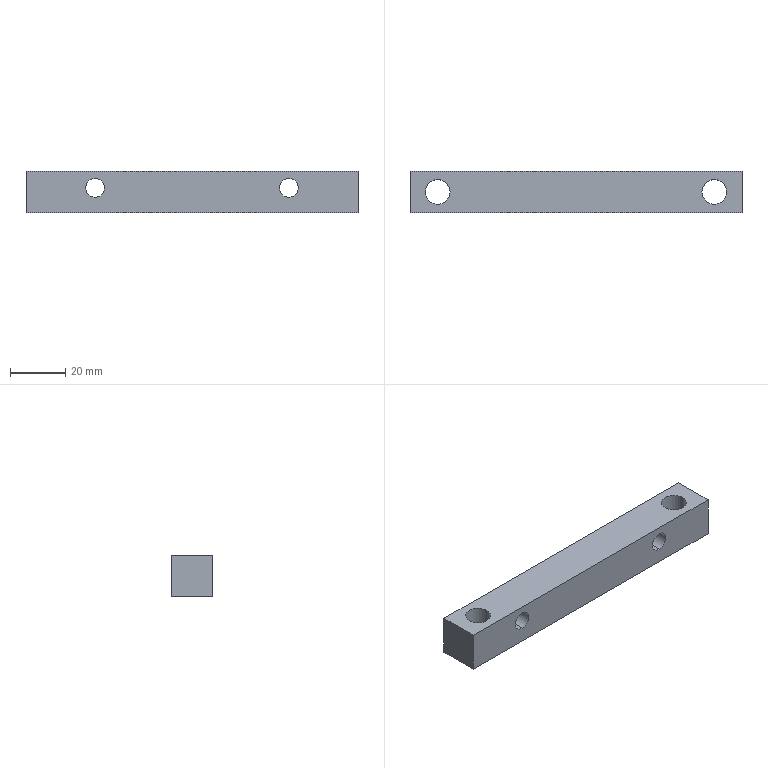Part | SolidWorks | features BaseBody 1 | 1 solid | 14 faces | box 120 x 15 x 15 mm | volume 24002 mm3 | cylinder 8 | plane 6 | commonest cylinder face diameters 6.8 x4 9 x4
STEP:
#1=CARTESIAN_POINT('',(-35.,7.5,12.4));
#2=VERTEX_POINT('',#1);
#3=CARTESIAN_POINT('',(-35.,7.5,5.6));
#4=VERTEX_POINT('',#3);
#5=CARTESIAN_POINT('',(-35.,7.5,9.));
#6=DIRECTION('',(0.,-1.,0.));
#7=DIRECTION('',(0.,0.,-1.));
#8=AXIS2_PLACEMENT_3D('',#5,#6,#7);
#9=CIRCLE('',#8,3.4);
#10=EDGE_CURVE('',#2,#4,#9,.T.);
#11=ORIENTED_EDGE('',*,*,#10,.F.);
#12=CARTESIAN_POINT('',(-35.,-7.5,12.4));
#13=VERTEX_POINT('',#12);
#14=CARTESIAN_POINT('',(-35.,-7.5,12.4));
#15=DIRECTION('',(0.,-1.,0.));
#16=VECTOR('',#15,1000.);
#17=LINE('',#14,#16);
#18=EDGE_CURVE('',#2,#13,#17,.T.);
#19=ORIENTED_EDGE('',*,*,#18,.T.);
#20=CARTESIAN_POINT('',(-35.,-7.5,5.6));
#21=VERTEX_POINT('',#20);
#22=CARTESIAN_POINT('',(-35.,-7.5,9.));
#23=DIRECTION('',(0.,-1.,0.));
#24=DIRECTION('',(0.,0.,-1.));
#25=AXIS2_PLACEMENT_3D('',#22,#23,#24);
#26=CIRCLE('',#25,3.4);
#27=EDGE_CURVE('',#13,#21,#26,.T.);
#28=ORIENTED_EDGE('',*,*,#27,.T.);
#29=CARTESIAN_POINT('',(-35.,-7.5,5.6));
#30=DIRECTION('',(0.,-1.,0.));
#31=VECTOR('',#30,1000.);
#32=LINE('',#29,#31);
#33=EDGE_CURVE('',#4,#21,#32,.T.);
#34=ORIENTED_EDGE('',*,*,#33,.F.);
#35=EDGE_LOOP('',(#11,#19,#28,#34));
#36=FACE_OUTER_BOUND('',#35,.T.);
#37=CARTESIAN_POINT('',(-35.,-7.5,9.));
#38=DIRECTION('',(0.,-1.,0.));
#39=DIRECTION('',(0.,0.,-1.));
#40=AXIS2_PLACEMENT_3D('',#37,#38,#39);
#41=CYLINDRICAL_SURFACE('',#40,3.4);
#42=ADVANCED_FACE('',(#36),#41,.F.);
#43=CARTESIAN_POINT('',(35.,7.5,12.4));
#44=VERTEX_POINT('',#43);
#45=CARTESIAN_POINT('',(35.,7.5,5.6));
#46=VERTEX_POINT('',#45);
#47=CARTESIAN_POINT('',(35.,7.5,9.));
#48=DIRECTION('',(0.,-1.,0.));
#49=DIRECTION('',(0.,0.,-1.));
#50=AXIS2_PLACEMENT_3D('',#47,#48,#49);
#51=CIRCLE('',#50,3.4);
#52=EDGE_CURVE('',#44,#46,#51,.T.);
#53=ORIENTED_EDGE('',*,*,#52,.F.);
#54=CARTESIAN_POINT('',(35.,-7.5,12.4));
#55=VERTEX_POINT('',#54);
#56=CARTESIAN_POINT('',(35.,-7.5,12.4));
#57=DIRECTION('',(0.,-1.,0.));
#58=VECTOR('',#57,1000.);
#59=LINE('',#56,#58);
#60=EDGE_CURVE('',#44,#55,#59,.T.);
#61=ORIENTED_EDGE('',*,*,#60,.T.);
#62=CARTESIAN_POINT('',(35.,-7.5,5.6));
#63=VERTEX_POINT('',#62);
#64=CARTESIAN_POINT('',(35.,-7.5,9.));
#65=DIRECTION('',(0.,-1.,0.));
#66=DIRECTION('',(0.,0.,-1.));
#67=AXIS2_PLACEMENT_3D('',#64,#65,#66);
#68=CIRCLE('',#67,3.4);
#69=EDGE_CURVE('',#55,#63,#68,.T.);
#70=ORIENTED_EDGE('',*,*,#69,.T.);
#71=CARTESIAN_POINT('',(35.,-7.5,5.6));
#72=DIRECTION('',(0.,-1.,0.));
#73=VECTOR('',#72,1000.);
#74=LINE('',#71,#73);
#75=EDGE_CURVE('',#46,#63,#74,.T.);
#76=ORIENTED_EDGE('',*,*,#75,.F.);
#77=EDGE_LOOP('',(#53,#61,#70,#76));
#78=FACE_OUTER_BOUND('',#77,.T.);
#79=CARTESIAN_POINT('',(35.,-7.5,9.));
#80=DIRECTION('',(0.,-1.,0.));
#81=DIRECTION('',(0.,0.,-1.));
#82=AXIS2_PLACEMENT_3D('',#79,#80,#81);
#83=CYLINDRICAL_SURFACE('',#82,3.4);
#84=ADVANCED_FACE('',(#78),#83,.F.);
#85=CARTESIAN_POINT('',(-54.5,0.,0.));
#86=VERTEX_POINT('',#85);
#87=CARTESIAN_POINT('',(-45.5,0.,0.));
#88=VERTEX_POINT('',#87);
#89=CARTESIAN_POINT('',(-50.,0.,0.));
#90=DIRECTION('',(0.,0.,1.));
#91=DIRECTION('',(1.,0.,0.));
#92=AXIS2_PLACEMENT_3D('',#89,#90,#91);
#93=CIRCLE('',#92,4.5);
#94=EDGE_CURVE('',#86,#88,#93,.T.);
#95=ORIENTED_EDGE('',*,*,#94,.F.);
#96=CARTESIAN_POINT('',(-54.5,0.,15.));
#97=VERTEX_POINT('',#96);
#98=CARTESIAN_POINT('',(-54.5,0.,15.));
#99=DIRECTION('',(0.,0.,1.));
#100=VECTOR('',#99,1000.);
#101=LINE('',#98,#100);
#102=EDGE_CURVE('',#86,#97,#101,.T.);
#103=ORIENTED_EDGE('',*,*,#102,.T.);
#104=CARTESIAN_POINT('',(-45.5,0.,15.));
#105=VERTEX_POINT('',#104);
#106=CARTESIAN_POINT('',(-50.,0.,15.));
#107=DIRECTION('',(0.,0.,1.));
#108=DIRECTION('',(1.,0.,0.));
#109=AXIS2_PLACEMENT_3D('',#106,#107,#108);
#110=CIRCLE('',#109,4.5);
#111=EDGE_CURVE('',#97,#105,#110,.T.);
#112=ORIENTED_EDGE('',*,*,#111,.T.);
#113=CARTESIAN_POINT('',(-45.5,0.,15.));
#114=DIRECTION('',(0.,0.,1.));
#115=VECTOR('',#114,1000.);
#116=LINE('',#113,#115);
#117=EDGE_CURVE('',#88,#105,#116,.T.);
#118=ORIENTED_EDGE('',*,*,#117,.F.);
#119=EDGE_LOOP('',(#95,#103,#112,#118));
#120=FACE_OUTER_BOUND('',#119,.T.);
#121=CARTESIAN_POINT('',(-50.,0.,15.));
#122=DIRECTION('',(0.,0.,1.));
#123=DIRECTION('',(1.,0.,0.));
#124=AXIS2_PLACEMENT_3D('',#121,#122,#123);
#125=CYLINDRICAL_SURFACE('',#124,4.5);
#126=ADVANCED_FACE('',(#120),#125,.F.);
#127=CARTESIAN_POINT('',(45.5,0.,0.));
#128=VERTEX_POINT('',#127);
#129=CARTESIAN_POINT('',(54.5,0.,0.));
#130=VERTEX_POINT('',#129);
#131=CARTESIAN_POINT('',(50.,0.,0.));
#132=DIRECTION('',(0.,0.,1.));
#133=DIRECTION('',(1.,0.,0.));
#134=AXIS2_PLACEMENT_3D('',#131,#132,#133);
#135=CIRCLE('',#134,4.5);
#136=EDGE_CURVE('',#128,#130,#135,.T.);
#137=ORIENTED_EDGE('',*,*,#136,.F.);
#138=CARTESIAN_POINT('',(45.5,0.,15.));
#139=VERTEX_POINT('',#138);
#140=CARTESIAN_POINT('',(45.5,0.,15.));
#141=DIRECTION('',(0.,0.,1.));
#142=VECTOR('',#141,1000.);
#143=LINE('',#140,#142);
#144=EDGE_CURVE('',#128,#139,#143,.T.);
#145=ORIENTED_EDGE('',*,*,#144,.T.);
#146=CARTESIAN_POINT('',(54.5,0.,15.));
#147=VERTEX_POINT('',#146);
#148=CARTESIAN_POINT('',(50.,0.,15.));
#149=DIRECTION('',(0.,0.,1.));
#150=DIRECTION('',(1.,0.,0.));
#151=AXIS2_PLACEMENT_3D('',#148,#149,#150);
#152=CIRCLE('',#151,4.5);
#153=EDGE_CURVE('',#139,#147,#152,.T.);
#154=ORIENTED_EDGE('',*,*,#153,.T.);
#155=CARTESIAN_POINT('',(54.5,0.,15.));
#156=DIRECTION('',(0.,0.,1.));
#157=VECTOR('',#156,1000.);
#158=LINE('',#155,#157);
#159=EDGE_CURVE('',#130,#147,#158,.T.);
#160=ORIENTED_EDGE('',*,*,#159,.F.);
#161=EDGE_LOOP('',(#137,#145,#154,#160));
#162=FACE_OUTER_BOUND('',#161,.T.);
#163=CARTESIAN_POINT('',(50.,0.,15.));
#164=DIRECTION('',(0.,0.,1.));
#165=DIRECTION('',(1.,0.,0.));
#166=AXIS2_PLACEMENT_3D('',#163,#164,#165);
#167=CYLINDRICAL_SURFACE('',#166,4.5);
#168=ADVANCED_FACE('',(#162),#167,.F.);
#169=CARTESIAN_POINT('',(60.,-7.5,0.));
#170=VERTEX_POINT('',#169);
#171=CARTESIAN_POINT('',(60.,7.5,0.));
#172=VERTEX_POINT('',#171);
#173=CARTESIAN_POINT('',(60.,7.5,0.));
#174=DIRECTION('',(0.,1.,0.));
#175=VECTOR('',#174,1000.);
#176=LINE('',#173,#175);
#177=EDGE_CURVE('',#170,#172,#176,.T.);
#178=ORIENTED_EDGE('',*,*,#177,.T.);
#179=CARTESIAN_POINT('',(60.,7.5,15.));
#180=VERTEX_POINT('',#179);
#181=CARTESIAN_POINT('',(60.,7.5,15.));
#182=DIRECTION('',(0.,0.,-1.));
#183=VECTOR('',#182,1000.);
#184=LINE('',#181,#183);
#185=EDGE_CURVE('',#180,#172,#184,.T.);
#186=ORIENTED_EDGE('',*,*,#185,.F.);
#187=CARTESIAN_POINT('',(60.,-7.5,15.));
#188=VERTEX_POINT('',#187);
#189=CARTESIAN_POINT('',(60.,7.5,15.));
#190=DIRECTION('',(0.,1.,0.));
#191=VECTOR('',#190,1000.);
#192=LINE('',#189,#191);
#193=EDGE_CURVE('',#188,#180,#192,.T.);
#194=ORIENTED_EDGE('',*,*,#193,.F.);
#195=CARTESIAN_POINT('',(60.,-7.5,15.));
#196=DIRECTION('',(0.,0.,-1.));
#197=VECTOR('',#196,1000.);
#198=LINE('',#195,#197);
#199=EDGE_CURVE('',#188,#170,#198,.T.);
#200=ORIENTED_EDGE('',*,*,#199,.T.);
#201=EDGE_LOOP('',(#178,#186,#194,#200));
#202=FACE_OUTER_BOUND('',#201,.T.);
#203=CARTESIAN_POINT('',(60.,7.5,15.));
#204=DIRECTION('',(-1.,0.,0.));
#205=DIRECTION('',(0.,0.,1.));
#206=AXIS2_PLACEMENT_3D('',#203,#204,#205);
#207=PLANE('',#206);
#208=ADVANCED_FACE('',(#202),#207,.F.);
#209=CARTESIAN_POINT('',(-35.,7.5,9.));
#210=DIRECTION('',(0.,-1.,0.));
#211=DIRECTION('',(0.,0.,-1.));
#212=AXIS2_PLACEMENT_3D('',#209,#210,#211);
#213=CIRCLE('',#212,3.4);
#214=EDGE_CURVE('',#4,#2,#213,.T.);
#215=ORIENTED_EDGE('',*,*,#214,.T.);
#216=ORIENTED_EDGE('',*,*,#10,.T.);
#217=EDGE_LOOP('',(#215,#216));
#218=FACE_BOUND('',#217,.T.);
#219=CARTESIAN_POINT('',(35.,7.5,9.));
#220=DIRECTION('',(0.,-1.,0.));
#221=DIRECTION('',(0.,0.,-1.));
#222=AXIS2_PLACEMENT_3D('',#219,#220,#221);
#223=CIRCLE('',#222,3.4);
#224=EDGE_CURVE('',#46,#44,#223,.T.);
#225=ORIENTED_EDGE('',*,*,#224,.T.);
#226=ORIENTED_EDGE('',*,*,#52,.T.);
#227=EDGE_LOOP('',(#225,#226));
#228=FACE_BOUND('',#227,.T.);
#229=CARTESIAN_POINT('',(-60.,7.5,0.));
#230=VERTEX_POINT('',#229);
#231=CARTESIAN_POINT('',(-60.,7.5,0.));
#232=DIRECTION('',(-1.,0.,0.));
#233=VECTOR('',#232,1000.);
#234=LINE('',#231,#233);
#235=EDGE_CURVE('',#172,#230,#234,.T.);
#236=ORIENTED_EDGE('',*,*,#235,.T.);
#237=CARTESIAN_POINT('',(-60.,7.5,15.));
#238=VERTEX_POINT('',#237);
#239=CARTESIAN_POINT('',(-60.,7.5,15.));
#240=DIRECTION('',(0.,0.,-1.));
#241=VECTOR('',#240,1000.);
#242=LINE('',#239,#241);
#243=EDGE_CURVE('',#238,#230,#242,.T.);
#244=ORIENTED_EDGE('',*,*,#243,.F.);
#245=CARTESIAN_POINT('',(-60.,7.5,15.));
#246=DIRECTION('',(-1.,0.,0.));
#247=VECTOR('',#246,1000.);
#248=LINE('',#245,#247);
#249=EDGE_CURVE('',#180,#238,#248,.T.);
#250=ORIENTED_EDGE('',*,*,#249,.F.);
#251=ORIENTED_EDGE('',*,*,#185,.T.);
#252=EDGE_LOOP('',(#236,#244,#250,#251));
#253=FACE_OUTER_BOUND('',#252,.T.);
#254=CARTESIAN_POINT('',(-60.,7.5,15.));
#255=DIRECTION('',(0.,-1.,0.));
#256=DIRECTION('',(0.,0.,-1.));
#257=AXIS2_PLACEMENT_3D('',#254,#255,#256);
#258=PLANE('',#257);
#259=ADVANCED_FACE('',(#218,#228,#253),#258,.F.);
#260=CARTESIAN_POINT('',(-60.,-7.5,0.));
#261=VERTEX_POINT('',#260);
#262=CARTESIAN_POINT('',(-60.,7.5,0.));
#263=DIRECTION('',(0.,-1.,0.));
#264=VECTOR('',#263,1000.);
#265=LINE('',#262,#264);
#266=EDGE_CURVE('',#230,#261,#265,.T.);
#267=ORIENTED_EDGE('',*,*,#266,.T.);
#268=CARTESIAN_POINT('',(-60.,-7.5,15.));
#269=VERTEX_POINT('',#268);
#270=CARTESIAN_POINT('',(-60.,-7.5,15.));
#271=DIRECTION('',(0.,0.,-1.));
#272=VECTOR('',#271,1000.);
#273=LINE('',#270,#272);
#274=EDGE_CURVE('',#269,#261,#273,.T.);
#275=ORIENTED_EDGE('',*,*,#274,.F.);
#276=CARTESIAN_POINT('',(-60.,7.5,15.));
#277=DIRECTION('',(0.,-1.,0.));
#278=VECTOR('',#277,1000.);
#279=LINE('',#276,#278);
#280=EDGE_CURVE('',#238,#269,#279,.T.);
#281=ORIENTED_EDGE('',*,*,#280,.F.);
#282=ORIENTED_EDGE('',*,*,#243,.T.);
#283=EDGE_LOOP('',(#267,#275,#281,#282));
#284=FACE_OUTER_BOUND('',#283,.T.);
#285=CARTESIAN_POINT('',(-60.,7.5,15.));
#286=DIRECTION('',(1.,0.,0.));
#287=DIRECTION('',(0.,0.,-1.));
#288=AXIS2_PLACEMENT_3D('',#285,#286,#287);
#289=PLANE('',#288);
#290=ADVANCED_FACE('',(#284),#289,.F.);
#291=CARTESIAN_POINT('',(-35.,-7.5,9.));
#292=DIRECTION('',(0.,-1.,0.));
#293=DIRECTION('',(0.,0.,-1.));
#294=AXIS2_PLACEMENT_3D('',#291,#292,#293);
#295=CIRCLE('',#294,3.4);
#296=EDGE_CURVE('',#21,#13,#295,.T.);
#297=ORIENTED_EDGE('',*,*,#296,.F.);
#298=ORIENTED_EDGE('',*,*,#27,.F.);
#299=EDGE_LOOP('',(#297,#298));
#300=FACE_BOUND('',#299,.T.);
#301=CARTESIAN_POINT('',(35.,-7.5,9.));
#302=DIRECTION('',(0.,-1.,0.));
#303=DIRECTION('',(0.,0.,-1.));
#304=AXIS2_PLACEMENT_3D('',#301,#302,#303);
#305=CIRCLE('',#304,3.4);
#306=EDGE_CURVE('',#63,#55,#305,.T.);
#307=ORIENTED_EDGE('',*,*,#306,.F.);
#308=ORIENTED_EDGE('',*,*,#69,.F.);
#309=EDGE_LOOP('',(#307,#308));
#310=FACE_BOUND('',#309,.T.);
#311=CARTESIAN_POINT('',(-60.,-7.5,0.));
#312=DIRECTION('',(1.,0.,0.));
#313=VECTOR('',#312,1000.);
#314=LINE('',#311,#313);
#315=EDGE_CURVE('',#261,#170,#314,.T.);
#316=ORIENTED_EDGE('',*,*,#315,.T.);
#317=ORIENTED_EDGE('',*,*,#199,.F.);
#318=CARTESIAN_POINT('',(-60.,-7.5,15.));
#319=DIRECTION('',(1.,0.,0.));
#320=VECTOR('',#319,1000.);
#321=LINE('',#318,#320);
#322=EDGE_CURVE('',#269,#188,#321,.T.);
#323=ORIENTED_EDGE('',*,*,#322,.F.);
#324=ORIENTED_EDGE('',*,*,#274,.T.);
#325=EDGE_LOOP('',(#316,#317,#323,#324));
#326=FACE_OUTER_BOUND('',#325,.T.);
#327=CARTESIAN_POINT('',(-60.,-7.5,15.));
#328=DIRECTION('',(0.,1.,0.));
#329=DIRECTION('',(0.,0.,1.));
#330=AXIS2_PLACEMENT_3D('',#327,#328,#329);
#331=PLANE('',#330);
#332=ADVANCED_FACE('',(#300,#310,#326),#331,.F.);
#333=CARTESIAN_POINT('',(-50.,0.,15.));
#334=DIRECTION('',(0.,0.,1.));
#335=DIRECTION('',(1.,0.,0.));
#336=AXIS2_PLACEMENT_3D('',#333,#334,#335);
#337=CIRCLE('',#336,4.5);
#338=EDGE_CURVE('',#105,#97,#337,.T.);
#339=ORIENTED_EDGE('',*,*,#338,.F.);
#340=ORIENTED_EDGE('',*,*,#111,.F.);
#341=EDGE_LOOP('',(#339,#340));
#342=FACE_BOUND('',#341,.T.);
#343=CARTESIAN_POINT('',(50.,0.,15.));
#344=DIRECTION('',(0.,0.,1.));
#345=DIRECTION('',(1.,0.,0.));
#346=AXIS2_PLACEMENT_3D('',#343,#344,#345);
#347=CIRCLE('',#346,4.5);
#348=EDGE_CURVE('',#147,#139,#347,.T.);
#349=ORIENTED_EDGE('',*,*,#348,.F.);
#350=ORIENTED_EDGE('',*,*,#153,.F.);
#351=EDGE_LOOP('',(#349,#350));
#352=FACE_BOUND('',#351,.T.);
#353=ORIENTED_EDGE('',*,*,#193,.T.);
#354=ORIENTED_EDGE('',*,*,#249,.T.);
#355=ORIENTED_EDGE('',*,*,#280,.T.);
#356=ORIENTED_EDGE('',*,*,#322,.T.);
#357=EDGE_LOOP('',(#353,#354,#355,#356));
#358=FACE_OUTER_BOUND('',#357,.T.);
#359=CARTESIAN_POINT('',(0.,0.,15.));
#360=DIRECTION('',(0.,0.,1.));
#361=DIRECTION('',(1.,0.,0.));
#362=AXIS2_PLACEMENT_3D('',#359,#360,#361);
#363=PLANE('',#362);
#364=ADVANCED_FACE('',(#342,#352,#358),#363,.T.);
#365=CARTESIAN_POINT('',(-50.,0.,0.));
#366=DIRECTION('',(0.,0.,1.));
#367=DIRECTION('',(1.,0.,0.));
#368=AXIS2_PLACEMENT_3D('',#365,#366,#367);
#369=CIRCLE('',#368,4.5);
#370=EDGE_CURVE('',#88,#86,#369,.T.);
#371=ORIENTED_EDGE('',*,*,#370,.T.);
#372=ORIENTED_EDGE('',*,*,#94,.T.);
#373=EDGE_LOOP('',(#371,#372));
#374=FACE_BOUND('',#373,.T.);
#375=CARTESIAN_POINT('',(50.,0.,0.));
#376=DIRECTION('',(0.,0.,1.));
#377=DIRECTION('',(1.,0.,0.));
#378=AXIS2_PLACEMENT_3D('',#375,#376,#377);
#379=CIRCLE('',#378,4.5);
#380=EDGE_CURVE('',#130,#128,#379,.T.);
#381=ORIENTED_EDGE('',*,*,#380,.T.);
#382=ORIENTED_EDGE('',*,*,#136,.T.);
#383=EDGE_LOOP('',(#381,#382));
#384=FACE_BOUND('',#383,.T.);
#385=ORIENTED_EDGE('',*,*,#177,.F.);
#386=ORIENTED_EDGE('',*,*,#315,.F.);
#387=ORIENTED_EDGE('',*,*,#266,.F.);
#388=ORIENTED_EDGE('',*,*,#235,.F.);
#389=EDGE_LOOP('',(#385,#386,#387,#388));
#390=FACE_OUTER_BOUND('',#389,.T.);
#391=CARTESIAN_POINT('',(0.,0.,0.));
#392=DIRECTION('',(0.,0.,1.));
#393=DIRECTION('',(1.,0.,0.));
#394=AXIS2_PLACEMENT_3D('',#391,#392,#393);
#395=PLANE('',#394);
#396=ADVANCED_FACE('',(#374,#384,#390),#395,.F.);
#397=ORIENTED_EDGE('',*,*,#144,.F.);
#398=ORIENTED_EDGE('',*,*,#380,.F.);
#399=ORIENTED_EDGE('',*,*,#159,.T.);
#400=ORIENTED_EDGE('',*,*,#348,.T.);
#401=EDGE_LOOP('',(#397,#398,#399,#400));
#402=FACE_OUTER_BOUND('',#401,.T.);
#403=CARTESIAN_POINT('',(50.,0.,15.));
#404=DIRECTION('',(0.,0.,1.));
#405=DIRECTION('',(1.,0.,0.));
#406=AXIS2_PLACEMENT_3D('',#403,#404,#405);
#407=CYLINDRICAL_SURFACE('',#406,4.5);
#408=ADVANCED_FACE('',(#402),#407,.F.);
#409=ORIENTED_EDGE('',*,*,#102,.F.);
#410=ORIENTED_EDGE('',*,*,#370,.F.);
#411=ORIENTED_EDGE('',*,*,#117,.T.);
#412=ORIENTED_EDGE('',*,*,#338,.T.);
#413=EDGE_LOOP('',(#409,#410,#411,#412));
#414=FACE_OUTER_BOUND('',#413,.T.);
#415=CARTESIAN_POINT('',(-50.,0.,15.));
#416=DIRECTION('',(0.,0.,1.));
#417=DIRECTION('',(1.,0.,0.));
#418=AXIS2_PLACEMENT_3D('',#415,#416,#417);
#419=CYLINDRICAL_SURFACE('',#418,4.5);
#420=ADVANCED_FACE('',(#414),#419,.F.);
#421=ORIENTED_EDGE('',*,*,#60,.F.);
#422=ORIENTED_EDGE('',*,*,#224,.F.);
#423=ORIENTED_EDGE('',*,*,#75,.T.);
#424=ORIENTED_EDGE('',*,*,#306,.T.);
#425=EDGE_LOOP('',(#421,#422,#423,#424));
#426=FACE_OUTER_BOUND('',#425,.T.);
#427=CARTESIAN_POINT('',(35.,-7.5,9.));
#428=DIRECTION('',(0.,-1.,0.));
#429=DIRECTION('',(0.,0.,-1.));
#430=AXIS2_PLACEMENT_3D('',#427,#428,#429);
#431=CYLINDRICAL_SURFACE('',#430,3.4);
#432=ADVANCED_FACE('',(#426),#431,.F.);
#433=ORIENTED_EDGE('',*,*,#18,.F.);
#434=ORIENTED_EDGE('',*,*,#214,.F.);
#435=ORIENTED_EDGE('',*,*,#33,.T.);
#436=ORIENTED_EDGE('',*,*,#296,.T.);
#437=EDGE_LOOP('',(#433,#434,#435,#436));
#438=FACE_OUTER_BOUND('',#437,.T.);
#439=CARTESIAN_POINT('',(-35.,-7.5,9.));
#440=DIRECTION('',(0.,-1.,0.));
#441=DIRECTION('',(0.,0.,-1.));
#442=AXIS2_PLACEMENT_3D('',#439,#440,#441);
#443=CYLINDRICAL_SURFACE('',#442,3.4);
#444=ADVANCED_FACE('',(#438),#443,.F.);
#445=CLOSED_SHELL('',(#42,#84,#126,#168,#208,#259,#290,#332,#364,#396,#408,#420,#432,#444));
#446=MANIFOLD_SOLID_BREP('',#445);
#447=CARTESIAN_POINT('',(0.,0.,0.));
#448=DIRECTION('',(0.,0.,1.));
#449=DIRECTION('',(1.,0.,0.));
#450=AXIS2_PLACEMENT_3D('',#447,#448,#449);
#451=(LENGTH_UNIT()NAMED_UNIT(*)SI_UNIT(.MILLI.,.METRE.));
#452=UNCERTAINTY_MEASURE_WITH_UNIT(LENGTH_MEASURE(0.00001),#451,'','');
#453=(NAMED_UNIT(*)PLANE_ANGLE_UNIT()SI_UNIT($,.RADIAN.));
#454=(NAMED_UNIT(*)SI_UNIT($,.STERADIAN.)SOLID_ANGLE_UNIT());
#455=(GEOMETRIC_REPRESENTATION_CONTEXT(3)GLOBAL_UNCERTAINTY_ASSIGNED_CONTEXT((#452))GLOBAL_UNIT_ASSIGNED_CONTEXT((#451,#453,#454))REPRESENTATION_CONTEXT('',''));
#456=ADVANCED_BREP_SHAPE_REPRESENTATION('',(#446,#450),#455);